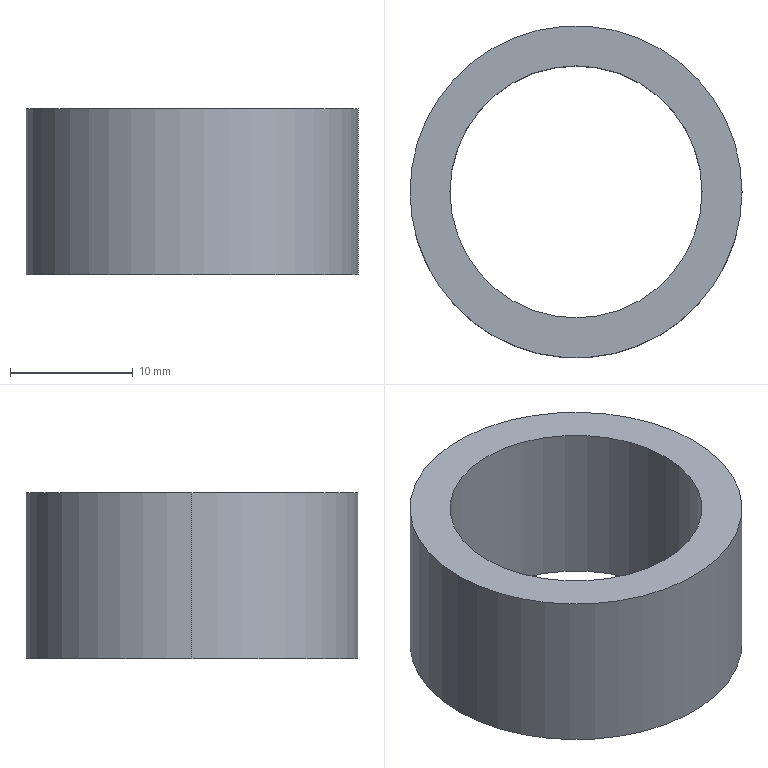Part | STEP file | 1 solid | 6 faces | box 27 x 27 x 13.5 mm | volume 3274 mm3 | cylinder 4 | plane 2 | commonest cylinder face diameters 20.5 x2 27 x2
STEP:
#1=CARTESIAN_POINT('',(0.,0.,0.));
#2=DIRECTION('',(0.,0.,1.));
#3=DIRECTION('',(1.,0.,0.));
#4=AXIS2_PLACEMENT_3D('',#1,#2,#3);
#5=CARTESIAN_POINT('',(10.25,0.,-6.75));
#6=VERTEX_POINT('',#5);
#7=CARTESIAN_POINT('',(-10.25,0.,-6.75));
#8=VERTEX_POINT('',#7);
#9=CARTESIAN_POINT('',(0.,0.,-6.75));
#10=DIRECTION('',(0.,0.,1.));
#11=DIRECTION('',(1.,0.,0.));
#12=AXIS2_PLACEMENT_3D('',#9,#10,#11);
#13=CIRCLE('',#12,10.25);
#14=CARTESIAN_POINT('',(0.,0.,6.75));
#15=DIRECTION('',(0.,0.,-1.));
#16=DIRECTION('',(-1.,0.,0.));
#17=AXIS2_PLACEMENT_3D('',#14,#15,#16);
#18=CYLINDRICAL_SURFACE('',#17,10.25);
#19=CARTESIAN_POINT('',(3.142,13.5));
#20=DIRECTION('',(-1.,0.));
#21=VECTOR('',#20,1.);
#22=LINE('',#19,#21);
#23=(GEOMETRIC_REPRESENTATION_CONTEXT(2)PARAMETRIC_REPRESENTATION_CONTEXT()REPRESENTATION_CONTEXT('',''));
#24=DEFINITIONAL_REPRESENTATION('',(#22),#23);
#25=PCURVE('',#18,#24);
#26=CARTESIAN_POINT('',(0.,0.,-6.75));
#27=DIRECTION('',(0.,0.,1.));
#28=DIRECTION('',(1.,0.,0.));
#29=AXIS2_PLACEMENT_3D('',#26,#27,#28);
#30=PLANE('',#29);
#31=CARTESIAN_POINT('',(0.,0.));
#32=DIRECTION('',(1.,0.));
#33=AXIS2_PLACEMENT_2D('',#31,#32);
#34=CIRCLE('',#33,10.25);
#35=(GEOMETRIC_REPRESENTATION_CONTEXT(2)PARAMETRIC_REPRESENTATION_CONTEXT()REPRESENTATION_CONTEXT('',''));
#36=DEFINITIONAL_REPRESENTATION('',(#34),#35);
#37=PCURVE('',#30,#36);
#38=SURFACE_CURVE('',#13,(#25,#37),.PCURVE_S1.);
#39=EDGE_CURVE('',#6,#8,#38,.T.);
#40=ORIENTED_EDGE('',*,*,#39,.T.);
#41=CARTESIAN_POINT('',(-10.25,0.,6.75));
#42=VERTEX_POINT('',#41);
#43=CARTESIAN_POINT('',(-10.25,0.,6.75));
#44=DIRECTION('',(0.,0.,-1.));
#45=VECTOR('',#44,1.);
#46=LINE('',#43,#45);
#47=CARTESIAN_POINT('',(0.,0.));
#48=DIRECTION('',(0.,1.));
#49=VECTOR('',#48,1.);
#50=LINE('',#47,#49);
#51=(GEOMETRIC_REPRESENTATION_CONTEXT(2)PARAMETRIC_REPRESENTATION_CONTEXT()REPRESENTATION_CONTEXT('',''));
#52=DEFINITIONAL_REPRESENTATION('',(#50),#51);
#53=PCURVE('',#18,#52);
#54=CARTESIAN_POINT('',(0.,0.,6.75));
#55=DIRECTION('',(0.,0.,-1.));
#56=DIRECTION('',(-1.,0.,0.));
#57=AXIS2_PLACEMENT_3D('',#54,#55,#56);
#58=CYLINDRICAL_SURFACE('',#57,10.25);
#59=CARTESIAN_POINT('',(6.283,0.));
#60=DIRECTION('',(0.,1.));
#61=VECTOR('',#60,1.);
#62=LINE('',#59,#61);
#63=(GEOMETRIC_REPRESENTATION_CONTEXT(2)PARAMETRIC_REPRESENTATION_CONTEXT()REPRESENTATION_CONTEXT('',''));
#64=DEFINITIONAL_REPRESENTATION('',(#62),#63);
#65=PCURVE('',#58,#64);
#66=SURFACE_CURVE('',#46,(#53,#65),.PCURVE_S1.);
#67=EDGE_CURVE('',#42,#8,#66,.T.);
#68=ORIENTED_EDGE('',*,*,#67,.F.);
#69=CARTESIAN_POINT('',(10.25,0.,6.75));
#70=VERTEX_POINT('',#69);
#71=CARTESIAN_POINT('',(0.,0.,6.75));
#72=DIRECTION('',(0.,0.,1.));
#73=DIRECTION('',(1.,0.,0.));
#74=AXIS2_PLACEMENT_3D('',#71,#72,#73);
#75=CIRCLE('',#74,10.25);
#76=CARTESIAN_POINT('',(3.142,0.));
#77=DIRECTION('',(-1.,0.));
#78=VECTOR('',#77,1.);
#79=LINE('',#76,#78);
#80=(GEOMETRIC_REPRESENTATION_CONTEXT(2)PARAMETRIC_REPRESENTATION_CONTEXT()REPRESENTATION_CONTEXT('',''));
#81=DEFINITIONAL_REPRESENTATION('',(#79),#80);
#82=PCURVE('',#18,#81);
#83=CARTESIAN_POINT('',(0.,0.,6.75));
#84=DIRECTION('',(0.,0.,1.));
#85=DIRECTION('',(1.,0.,0.));
#86=AXIS2_PLACEMENT_3D('',#83,#84,#85);
#87=PLANE('',#86);
#88=CARTESIAN_POINT('',(0.,0.));
#89=DIRECTION('',(1.,0.));
#90=AXIS2_PLACEMENT_2D('',#88,#89);
#91=CIRCLE('',#90,10.25);
#92=(GEOMETRIC_REPRESENTATION_CONTEXT(2)PARAMETRIC_REPRESENTATION_CONTEXT()REPRESENTATION_CONTEXT('',''));
#93=DEFINITIONAL_REPRESENTATION('',(#91),#92);
#94=PCURVE('',#87,#93);
#95=SURFACE_CURVE('',#75,(#82,#94),.PCURVE_S1.);
#96=EDGE_CURVE('',#70,#42,#95,.T.);
#97=ORIENTED_EDGE('',*,*,#96,.F.);
#98=CARTESIAN_POINT('',(10.25,0.,6.75));
#99=DIRECTION('',(0.,0.,-1.));
#100=VECTOR('',#99,1.);
#101=LINE('',#98,#100);
#102=CARTESIAN_POINT('',(3.142,0.));
#103=DIRECTION('',(0.,1.));
#104=VECTOR('',#103,1.);
#105=LINE('',#102,#104);
#106=(GEOMETRIC_REPRESENTATION_CONTEXT(2)PARAMETRIC_REPRESENTATION_CONTEXT()REPRESENTATION_CONTEXT('',''));
#107=DEFINITIONAL_REPRESENTATION('',(#105),#106);
#108=PCURVE('',#18,#107);
#109=CARTESIAN_POINT('',(3.142,0.));
#110=DIRECTION('',(0.,1.));
#111=VECTOR('',#110,1.);
#112=LINE('',#109,#111);
#113=(GEOMETRIC_REPRESENTATION_CONTEXT(2)PARAMETRIC_REPRESENTATION_CONTEXT()REPRESENTATION_CONTEXT('',''));
#114=DEFINITIONAL_REPRESENTATION('',(#112),#113);
#115=PCURVE('',#58,#114);
#116=SURFACE_CURVE('',#101,(#108,#115),.PCURVE_S1.);
#117=EDGE_CURVE('',#70,#6,#116,.T.);
#118=ORIENTED_EDGE('',*,*,#117,.T.);
#119=EDGE_LOOP('',(#40,#68,#97,#118));
#120=FACE_BOUND('',#119,.F.);
#121=ADVANCED_FACE('',(#120),#18,.F.);
#122=CARTESIAN_POINT('',(13.5,0.,6.75));
#123=VERTEX_POINT('',#122);
#124=CARTESIAN_POINT('',(13.5,0.,-6.75));
#125=VERTEX_POINT('',#124);
#126=CARTESIAN_POINT('',(13.5,0.,6.75));
#127=DIRECTION('',(0.,0.,-1.));
#128=VECTOR('',#127,1.);
#129=LINE('',#126,#128);
#130=CARTESIAN_POINT('',(0.,0.,6.75));
#131=DIRECTION('',(0.,0.,-1.));
#132=DIRECTION('',(-1.,0.,0.));
#133=AXIS2_PLACEMENT_3D('',#130,#131,#132);
#134=CYLINDRICAL_SURFACE('',#133,13.5);
#135=CARTESIAN_POINT('',(3.142,0.));
#136=DIRECTION('',(0.,1.));
#137=VECTOR('',#136,1.);
#138=LINE('',#135,#137);
#139=(GEOMETRIC_REPRESENTATION_CONTEXT(2)PARAMETRIC_REPRESENTATION_CONTEXT()REPRESENTATION_CONTEXT('',''));
#140=DEFINITIONAL_REPRESENTATION('',(#138),#139);
#141=PCURVE('',#134,#140);
#142=CARTESIAN_POINT('',(0.,0.,6.75));
#143=DIRECTION('',(0.,0.,-1.));
#144=DIRECTION('',(-1.,0.,0.));
#145=AXIS2_PLACEMENT_3D('',#142,#143,#144);
#146=CYLINDRICAL_SURFACE('',#145,13.5);
#147=CARTESIAN_POINT('',(3.142,0.));
#148=DIRECTION('',(0.,1.));
#149=VECTOR('',#148,1.);
#150=LINE('',#147,#149);
#151=(GEOMETRIC_REPRESENTATION_CONTEXT(2)PARAMETRIC_REPRESENTATION_CONTEXT()REPRESENTATION_CONTEXT('',''));
#152=DEFINITIONAL_REPRESENTATION('',(#150),#151);
#153=PCURVE('',#146,#152);
#154=SURFACE_CURVE('',#129,(#141,#153),.PCURVE_S1.);
#155=EDGE_CURVE('',#123,#125,#154,.T.);
#156=ORIENTED_EDGE('',*,*,#155,.F.);
#157=CARTESIAN_POINT('',(-13.5,0.,6.75));
#158=VERTEX_POINT('',#157);
#159=CARTESIAN_POINT('',(0.,0.,6.75));
#160=DIRECTION('',(0.,0.,1.));
#161=DIRECTION('',(1.,0.,0.));
#162=AXIS2_PLACEMENT_3D('',#159,#160,#161);
#163=CIRCLE('',#162,13.5);
#164=CARTESIAN_POINT('',(9.425,0.));
#165=DIRECTION('',(-1.,0.));
#166=VECTOR('',#165,1.);
#167=LINE('',#164,#166);
#168=(GEOMETRIC_REPRESENTATION_CONTEXT(2)PARAMETRIC_REPRESENTATION_CONTEXT()REPRESENTATION_CONTEXT('',''));
#169=DEFINITIONAL_REPRESENTATION('',(#167),#168);
#170=PCURVE('',#134,#169);
#171=CARTESIAN_POINT('',(0.,0.));
#172=DIRECTION('',(1.,0.));
#173=AXIS2_PLACEMENT_2D('',#171,#172);
#174=CIRCLE('',#173,13.5);
#175=(GEOMETRIC_REPRESENTATION_CONTEXT(2)PARAMETRIC_REPRESENTATION_CONTEXT()REPRESENTATION_CONTEXT('',''));
#176=DEFINITIONAL_REPRESENTATION('',(#174),#175);
#177=PCURVE('',#87,#176);
#178=SURFACE_CURVE('',#163,(#170,#177),.PCURVE_S1.);
#179=EDGE_CURVE('',#158,#123,#178,.T.);
#180=ORIENTED_EDGE('',*,*,#179,.F.);
#181=CARTESIAN_POINT('',(-13.5,0.,-6.75));
#182=VERTEX_POINT('',#181);
#183=CARTESIAN_POINT('',(-13.5,0.,6.75));
#184=DIRECTION('',(0.,0.,-1.));
#185=VECTOR('',#184,1.);
#186=LINE('',#183,#185);
#187=CARTESIAN_POINT('',(6.283,0.));
#188=DIRECTION('',(0.,1.));
#189=VECTOR('',#188,1.);
#190=LINE('',#187,#189);
#191=(GEOMETRIC_REPRESENTATION_CONTEXT(2)PARAMETRIC_REPRESENTATION_CONTEXT()REPRESENTATION_CONTEXT('',''));
#192=DEFINITIONAL_REPRESENTATION('',(#190),#191);
#193=PCURVE('',#134,#192);
#194=CARTESIAN_POINT('',(0.,0.));
#195=DIRECTION('',(0.,1.));
#196=VECTOR('',#195,1.);
#197=LINE('',#194,#196);
#198=(GEOMETRIC_REPRESENTATION_CONTEXT(2)PARAMETRIC_REPRESENTATION_CONTEXT()REPRESENTATION_CONTEXT('',''));
#199=DEFINITIONAL_REPRESENTATION('',(#197),#198);
#200=PCURVE('',#146,#199);
#201=SURFACE_CURVE('',#186,(#193,#200),.PCURVE_S1.);
#202=EDGE_CURVE('',#158,#182,#201,.T.);
#203=ORIENTED_EDGE('',*,*,#202,.T.);
#204=CARTESIAN_POINT('',(0.,0.,-6.75));
#205=DIRECTION('',(0.,0.,1.));
#206=DIRECTION('',(1.,0.,0.));
#207=AXIS2_PLACEMENT_3D('',#204,#205,#206);
#208=CIRCLE('',#207,13.5);
#209=CARTESIAN_POINT('',(9.425,13.5));
#210=DIRECTION('',(-1.,0.));
#211=VECTOR('',#210,1.);
#212=LINE('',#209,#211);
#213=(GEOMETRIC_REPRESENTATION_CONTEXT(2)PARAMETRIC_REPRESENTATION_CONTEXT()REPRESENTATION_CONTEXT('',''));
#214=DEFINITIONAL_REPRESENTATION('',(#212),#213);
#215=PCURVE('',#134,#214);
#216=CARTESIAN_POINT('',(0.,0.));
#217=DIRECTION('',(1.,0.));
#218=AXIS2_PLACEMENT_2D('',#216,#217);
#219=CIRCLE('',#218,13.5);
#220=(GEOMETRIC_REPRESENTATION_CONTEXT(2)PARAMETRIC_REPRESENTATION_CONTEXT()REPRESENTATION_CONTEXT('',''));
#221=DEFINITIONAL_REPRESENTATION('',(#219),#220);
#222=PCURVE('',#30,#221);
#223=SURFACE_CURVE('',#208,(#215,#222),.PCURVE_S1.);
#224=EDGE_CURVE('',#182,#125,#223,.T.);
#225=ORIENTED_EDGE('',*,*,#224,.T.);
#226=EDGE_LOOP('',(#156,#180,#203,#225));
#227=FACE_BOUND('',#226,.T.);
#228=ADVANCED_FACE('',(#227),#134,.T.);
#229=CARTESIAN_POINT('',(0.,0.,-6.75));
#230=DIRECTION('',(0.,0.,1.));
#231=DIRECTION('',(1.,0.,0.));
#232=AXIS2_PLACEMENT_3D('',#229,#230,#231);
#233=CIRCLE('',#232,10.25);
#234=CARTESIAN_POINT('',(0.,0.));
#235=DIRECTION('',(1.,0.));
#236=AXIS2_PLACEMENT_2D('',#234,#235);
#237=CIRCLE('',#236,10.25);
#238=(GEOMETRIC_REPRESENTATION_CONTEXT(2)PARAMETRIC_REPRESENTATION_CONTEXT()REPRESENTATION_CONTEXT('',''));
#239=DEFINITIONAL_REPRESENTATION('',(#237),#238);
#240=PCURVE('',#30,#239);
#241=CARTESIAN_POINT('',(9.425,13.5));
#242=DIRECTION('',(-1.,0.));
#243=VECTOR('',#242,1.);
#244=LINE('',#241,#243);
#245=(GEOMETRIC_REPRESENTATION_CONTEXT(2)PARAMETRIC_REPRESENTATION_CONTEXT()REPRESENTATION_CONTEXT('',''));
#246=DEFINITIONAL_REPRESENTATION('',(#244),#245);
#247=PCURVE('',#58,#246);
#248=SURFACE_CURVE('',#233,(#240,#247),.PCURVE_S1.);
#249=EDGE_CURVE('',#8,#6,#248,.T.);
#250=ORIENTED_EDGE('',*,*,#249,.T.);
#251=ORIENTED_EDGE('',*,*,#39,.T.);
#252=EDGE_LOOP('',(#250,#251));
#253=FACE_BOUND('',#252,.T.);
#254=ORIENTED_EDGE('',*,*,#224,.F.);
#255=CARTESIAN_POINT('',(0.,0.,-6.75));
#256=DIRECTION('',(0.,0.,1.));
#257=DIRECTION('',(1.,0.,0.));
#258=AXIS2_PLACEMENT_3D('',#255,#256,#257);
#259=CIRCLE('',#258,13.5);
#260=CARTESIAN_POINT('',(0.,0.));
#261=DIRECTION('',(1.,0.));
#262=AXIS2_PLACEMENT_2D('',#260,#261);
#263=CIRCLE('',#262,13.5);
#264=(GEOMETRIC_REPRESENTATION_CONTEXT(2)PARAMETRIC_REPRESENTATION_CONTEXT()REPRESENTATION_CONTEXT('',''));
#265=DEFINITIONAL_REPRESENTATION('',(#263),#264);
#266=PCURVE('',#30,#265);
#267=CARTESIAN_POINT('',(3.142,13.5));
#268=DIRECTION('',(-1.,0.));
#269=VECTOR('',#268,1.);
#270=LINE('',#267,#269);
#271=(GEOMETRIC_REPRESENTATION_CONTEXT(2)PARAMETRIC_REPRESENTATION_CONTEXT()REPRESENTATION_CONTEXT('',''));
#272=DEFINITIONAL_REPRESENTATION('',(#270),#271);
#273=PCURVE('',#146,#272);
#274=SURFACE_CURVE('',#259,(#266,#273),.PCURVE_S1.);
#275=EDGE_CURVE('',#125,#182,#274,.T.);
#276=ORIENTED_EDGE('',*,*,#275,.F.);
#277=EDGE_LOOP('',(#254,#276));
#278=FACE_BOUND('',#277,.T.);
#279=ADVANCED_FACE('',(#253,#278),#30,.F.);
#280=CARTESIAN_POINT('',(0.,0.,6.75));
#281=DIRECTION('',(0.,0.,1.));
#282=DIRECTION('',(1.,0.,0.));
#283=AXIS2_PLACEMENT_3D('',#280,#281,#282);
#284=CIRCLE('',#283,10.25);
#285=CARTESIAN_POINT('',(0.,0.));
#286=DIRECTION('',(1.,0.));
#287=AXIS2_PLACEMENT_2D('',#285,#286);
#288=CIRCLE('',#287,10.25);
#289=(GEOMETRIC_REPRESENTATION_CONTEXT(2)PARAMETRIC_REPRESENTATION_CONTEXT()REPRESENTATION_CONTEXT('',''));
#290=DEFINITIONAL_REPRESENTATION('',(#288),#289);
#291=PCURVE('',#87,#290);
#292=CARTESIAN_POINT('',(9.425,0.));
#293=DIRECTION('',(-1.,0.));
#294=VECTOR('',#293,1.);
#295=LINE('',#292,#294);
#296=(GEOMETRIC_REPRESENTATION_CONTEXT(2)PARAMETRIC_REPRESENTATION_CONTEXT()REPRESENTATION_CONTEXT('',''));
#297=DEFINITIONAL_REPRESENTATION('',(#295),#296);
#298=PCURVE('',#58,#297);
#299=SURFACE_CURVE('',#284,(#291,#298),.PCURVE_S1.);
#300=EDGE_CURVE('',#42,#70,#299,.T.);
#301=ORIENTED_EDGE('',*,*,#300,.F.);
#302=ORIENTED_EDGE('',*,*,#96,.F.);
#303=EDGE_LOOP('',(#301,#302));
#304=FACE_BOUND('',#303,.T.);
#305=ORIENTED_EDGE('',*,*,#179,.T.);
#306=CARTESIAN_POINT('',(0.,0.,6.75));
#307=DIRECTION('',(0.,0.,1.));
#308=DIRECTION('',(1.,0.,0.));
#309=AXIS2_PLACEMENT_3D('',#306,#307,#308);
#310=CIRCLE('',#309,13.5);
#311=CARTESIAN_POINT('',(0.,0.));
#312=DIRECTION('',(1.,0.));
#313=AXIS2_PLACEMENT_2D('',#311,#312);
#314=CIRCLE('',#313,13.5);
#315=(GEOMETRIC_REPRESENTATION_CONTEXT(2)PARAMETRIC_REPRESENTATION_CONTEXT()REPRESENTATION_CONTEXT('',''));
#316=DEFINITIONAL_REPRESENTATION('',(#314),#315);
#317=PCURVE('',#87,#316);
#318=CARTESIAN_POINT('',(3.142,0.));
#319=DIRECTION('',(-1.,0.));
#320=VECTOR('',#319,1.);
#321=LINE('',#318,#320);
#322=(GEOMETRIC_REPRESENTATION_CONTEXT(2)PARAMETRIC_REPRESENTATION_CONTEXT()REPRESENTATION_CONTEXT('',''));
#323=DEFINITIONAL_REPRESENTATION('',(#321),#322);
#324=PCURVE('',#146,#323);
#325=SURFACE_CURVE('',#310,(#317,#324),.PCURVE_S1.);
#326=EDGE_CURVE('',#123,#158,#325,.T.);
#327=ORIENTED_EDGE('',*,*,#326,.T.);
#328=EDGE_LOOP('',(#305,#327));
#329=FACE_BOUND('',#328,.T.);
#330=ADVANCED_FACE('',(#304,#329),#87,.T.);
#331=ORIENTED_EDGE('',*,*,#326,.F.);
#332=ORIENTED_EDGE('',*,*,#155,.T.);
#333=ORIENTED_EDGE('',*,*,#275,.T.);
#334=ORIENTED_EDGE('',*,*,#202,.F.);
#335=EDGE_LOOP('',(#331,#332,#333,#334));
#336=FACE_BOUND('',#335,.T.);
#337=ADVANCED_FACE('',(#336),#146,.T.);
#338=ORIENTED_EDGE('',*,*,#67,.T.);
#339=ORIENTED_EDGE('',*,*,#249,.T.);
#340=ORIENTED_EDGE('',*,*,#117,.F.);
#341=ORIENTED_EDGE('',*,*,#300,.F.);
#342=EDGE_LOOP('',(#338,#339,#340,#341));
#343=FACE_BOUND('',#342,.F.);
#344=ADVANCED_FACE('',(#343),#58,.F.);
#345=CLOSED_SHELL('',(#121,#228,#279,#330,#337,#344));
#346=MANIFOLD_SOLID_BREP('',#345);
#347=(LENGTH_UNIT()NAMED_UNIT(*)SI_UNIT(.MILLI.,.METRE.));
#348=UNCERTAINTY_MEASURE_WITH_UNIT(LENGTH_MEASURE(0.0000001),#347,'','');
#349=(NAMED_UNIT(*)PLANE_ANGLE_UNIT()SI_UNIT($,.RADIAN.));
#350=(NAMED_UNIT(*)SI_UNIT($,.STERADIAN.)SOLID_ANGLE_UNIT());
#351=(GEOMETRIC_REPRESENTATION_CONTEXT(3)GLOBAL_UNCERTAINTY_ASSIGNED_CONTEXT((#348))GLOBAL_UNIT_ASSIGNED_CONTEXT((#347,#349,#350))REPRESENTATION_CONTEXT('',''));
#352=ADVANCED_BREP_SHAPE_REPRESENTATION('',(#4,#346),#351);